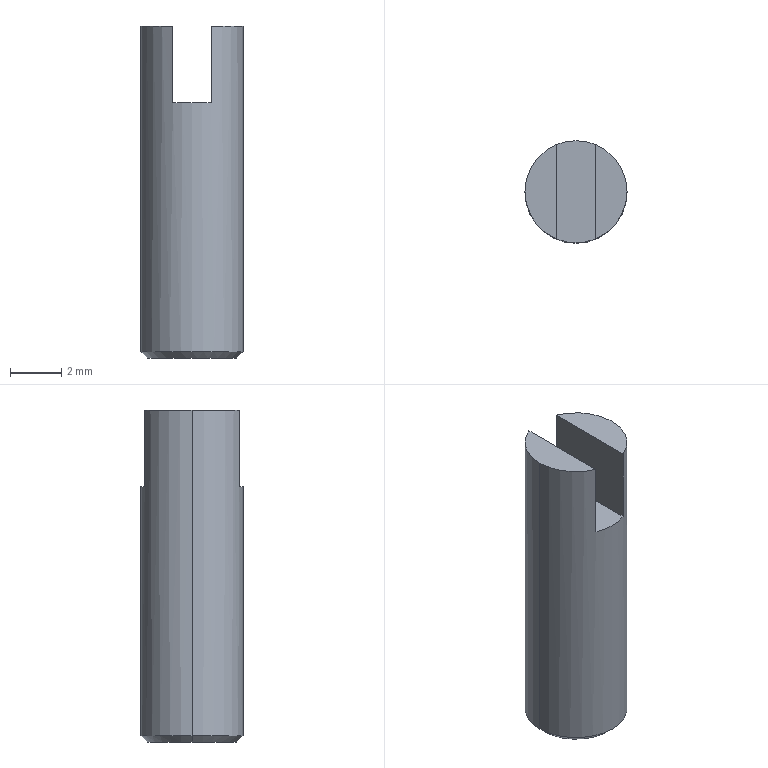Part | SolidWorks | features BaseBody 1 | 1 solid | 10 faces | box 4 x 4 x 13 mm | volume 145.418 mm3 | plane 6 | cone 2 | cylinder 2 | commonest cylinder face diameters 4 x2
STEP:
#1=CARTESIAN_POINT('',(-1.75,0.,0.));
#2=VERTEX_POINT('',#1);
#3=CARTESIAN_POINT('',(1.75,0.,0.));
#4=VERTEX_POINT('',#3);
#5=CARTESIAN_POINT('',(0.,0.,0.));
#6=DIRECTION('',(0.,0.,1.));
#7=DIRECTION('',(-1.,0.,0.));
#8=AXIS2_PLACEMENT_3D('',#5,#6,#7);
#9=CIRCLE('',#8,1.75);
#10=EDGE_CURVE('',#2,#4,#9,.T.);
#11=ORIENTED_EDGE('',*,*,#10,.T.);
#12=CARTESIAN_POINT('',(2.,0.,0.25));
#13=VERTEX_POINT('',#12);
#14=CARTESIAN_POINT('',(1.875,0.,0.125));
#15=DIRECTION('',(0.7071,0.,0.7071));
#16=VECTOR('',#15,1000.);
#17=LINE('',#14,#16);
#18=EDGE_CURVE('',#4,#13,#17,.T.);
#19=ORIENTED_EDGE('',*,*,#18,.T.);
#20=CARTESIAN_POINT('',(-2.,0.,0.25));
#21=VERTEX_POINT('',#20);
#22=CARTESIAN_POINT('',(0.,0.,0.25));
#23=DIRECTION('',(0.,0.,-1.));
#24=DIRECTION('',(-1.,0.,0.));
#25=AXIS2_PLACEMENT_3D('',#22,#23,#24);
#26=CIRCLE('',#25,2.);
#27=EDGE_CURVE('',#13,#21,#26,.T.);
#28=ORIENTED_EDGE('',*,*,#27,.T.);
#29=CARTESIAN_POINT('',(-1.875,0.,0.125));
#30=DIRECTION('',(-0.7071,0.,0.7071));
#31=VECTOR('',#30,1000.);
#32=LINE('',#29,#31);
#33=EDGE_CURVE('',#2,#21,#32,.T.);
#34=ORIENTED_EDGE('',*,*,#33,.F.);
#35=EDGE_LOOP('',(#11,#19,#28,#34));
#36=FACE_OUTER_BOUND('',#35,.T.);
#37=CARTESIAN_POINT('',(0.,0.,0.125));
#38=DIRECTION('',(0.,0.,1.));
#39=DIRECTION('',(-1.,0.,0.));
#40=AXIS2_PLACEMENT_3D('',#37,#38,#39);
#41=CONICAL_SURFACE('',#40,1.875,0.7854);
#42=ADVANCED_FACE('',(#36),#41,.T.);
#43=CARTESIAN_POINT('',(2.,0.,13.));
#44=VERTEX_POINT('',#43);
#45=CARTESIAN_POINT('',(0.75,1.854,13.));
#46=VERTEX_POINT('',#45);
#47=CARTESIAN_POINT('',(0.,0.,13.));
#48=DIRECTION('',(0.,0.,1.));
#49=DIRECTION('',(-1.,0.,0.));
#50=AXIS2_PLACEMENT_3D('',#47,#48,#49);
#51=CIRCLE('',#50,2.);
#52=EDGE_CURVE('',#44,#46,#51,.T.);
#53=ORIENTED_EDGE('',*,*,#52,.F.);
#54=CARTESIAN_POINT('',(2.,0.,0.));
#55=DIRECTION('',(0.,0.,-1.));
#56=VECTOR('',#55,1000.);
#57=LINE('',#54,#56);
#58=EDGE_CURVE('',#44,#13,#57,.T.);
#59=ORIENTED_EDGE('',*,*,#58,.T.);
#60=CARTESIAN_POINT('',(0.,0.,0.25));
#61=DIRECTION('',(0.,0.,-1.));
#62=DIRECTION('',(-1.,0.,0.));
#63=AXIS2_PLACEMENT_3D('',#60,#61,#62);
#64=CIRCLE('',#63,2.);
#65=EDGE_CURVE('',#21,#13,#64,.T.);
#66=ORIENTED_EDGE('',*,*,#65,.F.);
#67=CARTESIAN_POINT('',(-2.,0.,13.));
#68=VERTEX_POINT('',#67);
#69=CARTESIAN_POINT('',(-2.,0.,0.));
#70=DIRECTION('',(0.,0.,-1.));
#71=VECTOR('',#70,1000.);
#72=LINE('',#69,#71);
#73=EDGE_CURVE('',#68,#21,#72,.T.);
#74=ORIENTED_EDGE('',*,*,#73,.F.);
#75=CARTESIAN_POINT('',(-0.75,1.854,13.));
#76=VERTEX_POINT('',#75);
#77=CARTESIAN_POINT('',(0.,0.,13.));
#78=DIRECTION('',(0.,0.,1.));
#79=DIRECTION('',(-1.,0.,0.));
#80=AXIS2_PLACEMENT_3D('',#77,#78,#79);
#81=CIRCLE('',#80,2.);
#82=EDGE_CURVE('',#76,#68,#81,.T.);
#83=ORIENTED_EDGE('',*,*,#82,.F.);
#84=CARTESIAN_POINT('',(-0.75,1.854,10.));
#85=VERTEX_POINT('',#84);
#86=CARTESIAN_POINT('',(-0.75,1.854,0.));
#87=DIRECTION('',(0.,0.,-1.));
#88=VECTOR('',#87,1000.);
#89=LINE('',#86,#88);
#90=EDGE_CURVE('',#76,#85,#89,.T.);
#91=ORIENTED_EDGE('',*,*,#90,.T.);
#92=CARTESIAN_POINT('',(0.75,1.854,10.));
#93=VERTEX_POINT('',#92);
#94=CARTESIAN_POINT('',(0.,0.,10.));
#95=DIRECTION('',(0.,0.,-1.));
#96=DIRECTION('',(-1.,0.,0.));
#97=AXIS2_PLACEMENT_3D('',#94,#95,#96);
#98=CIRCLE('',#97,2.);
#99=EDGE_CURVE('',#85,#93,#98,.T.);
#100=ORIENTED_EDGE('',*,*,#99,.T.);
#101=CARTESIAN_POINT('',(0.75,1.854,0.));
#102=DIRECTION('',(0.,0.,1.));
#103=VECTOR('',#102,1000.);
#104=LINE('',#101,#103);
#105=EDGE_CURVE('',#93,#46,#104,.T.);
#106=ORIENTED_EDGE('',*,*,#105,.T.);
#107=EDGE_LOOP('',(#53,#59,#66,#74,#83,#91,#100,#106));
#108=FACE_OUTER_BOUND('',#107,.T.);
#109=CARTESIAN_POINT('',(0.,0.,0.));
#110=DIRECTION('',(0.,0.,-1.));
#111=DIRECTION('',(-1.,0.,0.));
#112=AXIS2_PLACEMENT_3D('',#109,#110,#111);
#113=CYLINDRICAL_SURFACE('',#112,2.);
#114=ADVANCED_FACE('',(#108),#113,.T.);
#115=ORIENTED_EDGE('',*,*,#10,.F.);
#116=CARTESIAN_POINT('',(0.,0.,0.));
#117=DIRECTION('',(0.,0.,1.));
#118=DIRECTION('',(-1.,0.,0.));
#119=AXIS2_PLACEMENT_3D('',#116,#117,#118);
#120=CIRCLE('',#119,1.75);
#121=EDGE_CURVE('',#4,#2,#120,.T.);
#122=ORIENTED_EDGE('',*,*,#121,.F.);
#123=EDGE_LOOP('',(#115,#122));
#124=FACE_OUTER_BOUND('',#123,.T.);
#125=CARTESIAN_POINT('',(0.,0.,0.));
#126=DIRECTION('',(0.,0.,1.));
#127=DIRECTION('',(1.,0.,0.));
#128=AXIS2_PLACEMENT_3D('',#125,#126,#127);
#129=PLANE('',#128);
#130=ADVANCED_FACE('',(#124),#129,.F.);
#131=CARTESIAN_POINT('',(-0.75,-1.854,10.));
#132=VERTEX_POINT('',#131);
#133=CARTESIAN_POINT('',(-0.75,-1.854,13.));
#134=VERTEX_POINT('',#133);
#135=CARTESIAN_POINT('',(-0.75,-1.854,0.));
#136=DIRECTION('',(0.,0.,1.));
#137=VECTOR('',#136,1000.);
#138=LINE('',#135,#137);
#139=EDGE_CURVE('',#132,#134,#138,.T.);
#140=ORIENTED_EDGE('',*,*,#139,.F.);
#141=CARTESIAN_POINT('',(-0.75,-2.,10.));
#142=DIRECTION('',(0.,1.,0.));
#143=VECTOR('',#142,1000.);
#144=LINE('',#141,#143);
#145=EDGE_CURVE('',#132,#85,#144,.T.);
#146=ORIENTED_EDGE('',*,*,#145,.T.);
#147=ORIENTED_EDGE('',*,*,#90,.F.);
#148=CARTESIAN_POINT('',(-0.75,-1.,13.));
#149=DIRECTION('',(0.,1.,0.));
#150=VECTOR('',#149,1000.);
#151=LINE('',#148,#150);
#152=EDGE_CURVE('',#134,#76,#151,.T.);
#153=ORIENTED_EDGE('',*,*,#152,.F.);
#154=EDGE_LOOP('',(#140,#146,#147,#153));
#155=FACE_OUTER_BOUND('',#154,.T.);
#156=CARTESIAN_POINT('',(-0.75,-2.,13.));
#157=DIRECTION('',(-1.,0.,0.));
#158=DIRECTION('',(0.,1.,0.));
#159=AXIS2_PLACEMENT_3D('',#156,#157,#158);
#160=PLANE('',#159);
#161=ADVANCED_FACE('',(#155),#160,.F.);
#162=CARTESIAN_POINT('',(0.75,-1.854,10.));
#163=VERTEX_POINT('',#162);
#164=CARTESIAN_POINT('',(0.,0.,10.));
#165=DIRECTION('',(0.,0.,-1.));
#166=DIRECTION('',(-1.,0.,0.));
#167=AXIS2_PLACEMENT_3D('',#164,#165,#166);
#168=CIRCLE('',#167,2.);
#169=EDGE_CURVE('',#163,#132,#168,.T.);
#170=ORIENTED_EDGE('',*,*,#169,.F.);
#171=CARTESIAN_POINT('',(0.75,2.,10.));
#172=DIRECTION('',(0.,-1.,0.));
#173=VECTOR('',#172,1000.);
#174=LINE('',#171,#173);
#175=EDGE_CURVE('',#93,#163,#174,.T.);
#176=ORIENTED_EDGE('',*,*,#175,.F.);
#177=ORIENTED_EDGE('',*,*,#99,.F.);
#178=ORIENTED_EDGE('',*,*,#145,.F.);
#179=EDGE_LOOP('',(#170,#176,#177,#178));
#180=FACE_OUTER_BOUND('',#179,.T.);
#181=CARTESIAN_POINT('',(0.,0.,10.));
#182=DIRECTION('',(0.,0.,-1.));
#183=DIRECTION('',(0.,-1.,0.));
#184=AXIS2_PLACEMENT_3D('',#181,#182,#183);
#185=PLANE('',#184);
#186=ADVANCED_FACE('',(#180),#185,.F.);
#187=CARTESIAN_POINT('',(0.75,-1.854,13.));
#188=VERTEX_POINT('',#187);
#189=CARTESIAN_POINT('',(0.75,-1.854,0.));
#190=DIRECTION('',(0.,0.,-1.));
#191=VECTOR('',#190,1000.);
#192=LINE('',#189,#191);
#193=EDGE_CURVE('',#188,#163,#192,.T.);
#194=ORIENTED_EDGE('',*,*,#193,.F.);
#195=CARTESIAN_POINT('',(0.75,1.,13.));
#196=DIRECTION('',(0.,-1.,0.));
#197=VECTOR('',#196,1000.);
#198=LINE('',#195,#197);
#199=EDGE_CURVE('',#46,#188,#198,.T.);
#200=ORIENTED_EDGE('',*,*,#199,.F.);
#201=ORIENTED_EDGE('',*,*,#105,.F.);
#202=ORIENTED_EDGE('',*,*,#175,.T.);
#203=EDGE_LOOP('',(#194,#200,#201,#202));
#204=FACE_OUTER_BOUND('',#203,.T.);
#205=CARTESIAN_POINT('',(0.75,2.,13.));
#206=DIRECTION('',(1.,0.,0.));
#207=DIRECTION('',(0.,-1.,0.));
#208=AXIS2_PLACEMENT_3D('',#205,#206,#207);
#209=PLANE('',#208);
#210=ADVANCED_FACE('',(#204),#209,.F.);
#211=ORIENTED_EDGE('',*,*,#152,.T.);
#212=ORIENTED_EDGE('',*,*,#82,.T.);
#213=CARTESIAN_POINT('',(0.,0.,13.));
#214=DIRECTION('',(0.,0.,1.));
#215=DIRECTION('',(-1.,0.,0.));
#216=AXIS2_PLACEMENT_3D('',#213,#214,#215);
#217=CIRCLE('',#216,2.);
#218=EDGE_CURVE('',#68,#134,#217,.T.);
#219=ORIENTED_EDGE('',*,*,#218,.T.);
#220=EDGE_LOOP('',(#211,#212,#219));
#221=FACE_OUTER_BOUND('',#220,.T.);
#222=CARTESIAN_POINT('',(0.,0.,13.));
#223=DIRECTION('',(0.,0.,1.));
#224=DIRECTION('',(1.,0.,0.));
#225=AXIS2_PLACEMENT_3D('',#222,#223,#224);
#226=PLANE('',#225);
#227=ADVANCED_FACE('',(#221),#226,.T.);
#228=ORIENTED_EDGE('',*,*,#199,.T.);
#229=CARTESIAN_POINT('',(0.,0.,13.));
#230=DIRECTION('',(0.,0.,1.));
#231=DIRECTION('',(-1.,0.,0.));
#232=AXIS2_PLACEMENT_3D('',#229,#230,#231);
#233=CIRCLE('',#232,2.);
#234=EDGE_CURVE('',#188,#44,#233,.T.);
#235=ORIENTED_EDGE('',*,*,#234,.T.);
#236=ORIENTED_EDGE('',*,*,#52,.T.);
#237=EDGE_LOOP('',(#228,#235,#236));
#238=FACE_OUTER_BOUND('',#237,.T.);
#239=CARTESIAN_POINT('',(0.,0.,13.));
#240=DIRECTION('',(0.,0.,1.));
#241=DIRECTION('',(1.,0.,0.));
#242=AXIS2_PLACEMENT_3D('',#239,#240,#241);
#243=PLANE('',#242);
#244=ADVANCED_FACE('',(#238),#243,.T.);
#245=ORIENTED_EDGE('',*,*,#58,.F.);
#246=ORIENTED_EDGE('',*,*,#234,.F.);
#247=ORIENTED_EDGE('',*,*,#193,.T.);
#248=ORIENTED_EDGE('',*,*,#169,.T.);
#249=ORIENTED_EDGE('',*,*,#139,.T.);
#250=ORIENTED_EDGE('',*,*,#218,.F.);
#251=ORIENTED_EDGE('',*,*,#73,.T.);
#252=ORIENTED_EDGE('',*,*,#27,.F.);
#253=EDGE_LOOP('',(#245,#246,#247,#248,#249,#250,#251,#252));
#254=FACE_OUTER_BOUND('',#253,.T.);
#255=CARTESIAN_POINT('',(0.,0.,0.));
#256=DIRECTION('',(0.,0.,-1.));
#257=DIRECTION('',(-1.,0.,0.));
#258=AXIS2_PLACEMENT_3D('',#255,#256,#257);
#259=CYLINDRICAL_SURFACE('',#258,2.);
#260=ADVANCED_FACE('',(#254),#259,.T.);
#261=ORIENTED_EDGE('',*,*,#18,.F.);
#262=ORIENTED_EDGE('',*,*,#121,.T.);
#263=ORIENTED_EDGE('',*,*,#33,.T.);
#264=ORIENTED_EDGE('',*,*,#65,.T.);
#265=EDGE_LOOP('',(#261,#262,#263,#264));
#266=FACE_OUTER_BOUND('',#265,.T.);
#267=CARTESIAN_POINT('',(0.,0.,0.125));
#268=DIRECTION('',(0.,0.,1.));
#269=DIRECTION('',(-1.,0.,0.));
#270=AXIS2_PLACEMENT_3D('',#267,#268,#269);
#271=CONICAL_SURFACE('',#270,1.875,0.7854);
#272=ADVANCED_FACE('',(#266),#271,.T.);
#273=CLOSED_SHELL('',(#42,#114,#130,#161,#186,#210,#227,#244,#260,#272));
#274=MANIFOLD_SOLID_BREP('',#273);
#275=CARTESIAN_POINT('',(0.,0.,0.));
#276=DIRECTION('',(0.,0.,1.));
#277=DIRECTION('',(1.,0.,0.));
#278=AXIS2_PLACEMENT_3D('',#275,#276,#277);
#279=(LENGTH_UNIT()NAMED_UNIT(*)SI_UNIT(.MILLI.,.METRE.));
#280=UNCERTAINTY_MEASURE_WITH_UNIT(LENGTH_MEASURE(0.00001),#279,'','');
#281=(NAMED_UNIT(*)PLANE_ANGLE_UNIT()SI_UNIT($,.RADIAN.));
#282=(NAMED_UNIT(*)SI_UNIT($,.STERADIAN.)SOLID_ANGLE_UNIT());
#283=(GEOMETRIC_REPRESENTATION_CONTEXT(3)GLOBAL_UNCERTAINTY_ASSIGNED_CONTEXT((#280))GLOBAL_UNIT_ASSIGNED_CONTEXT((#279,#281,#282))REPRESENTATION_CONTEXT('',''));
#284=ADVANCED_BREP_SHAPE_REPRESENTATION('',(#274,#278),#283);